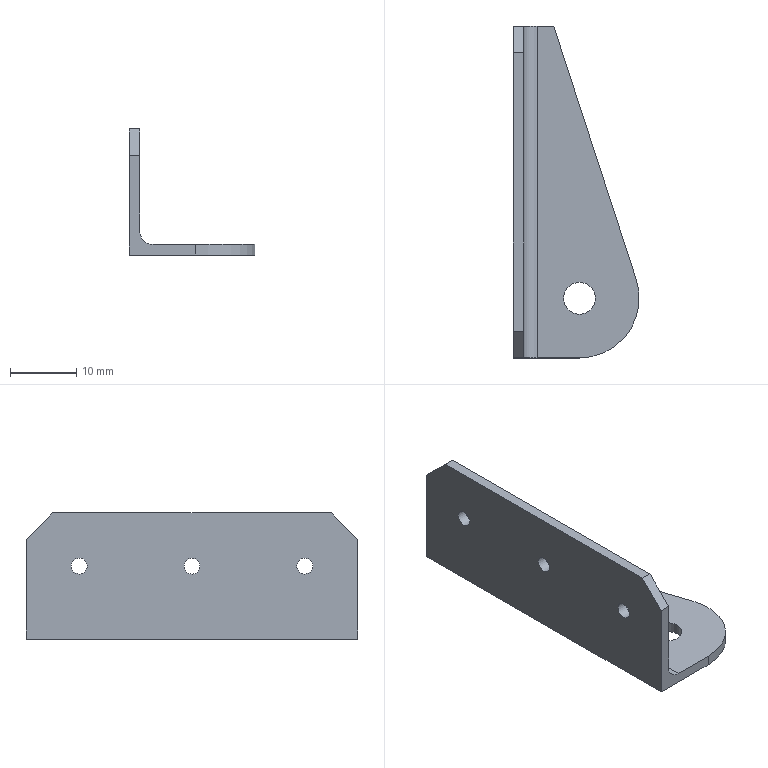Part | NX | features solid 2 | 1 solid | 16 faces | box 18.999 x 50 x 19 mm | volume 2444 mm3 | plane 10 | cylinder 6 | commonest cylinder face diameters 2.4 x3 4 x1 4.8 x1 17.997 x1
STEP:
#1=CARTESIAN_POINT('',(108.762,-251.916,9.8));
#2=VERTEX_POINT('',#1);
#3=CARTESIAN_POINT('',(108.762,-251.916,11.));
#4=DIRECTION('',(1.,0.,0.));
#5=DIRECTION('',(0.,0.,-1.));
#6=AXIS2_PLACEMENT_3D('',#3,#4,#5);
#7=CIRCLE('',#6,1.2);
#8=EDGE_CURVE('',#2,#2,#7,.F.);
#9=ORIENTED_EDGE('',*,*,#8,.F.);
#10=EDGE_LOOP('',(#9));
#11=FACE_BOUND('',#10,.T.);
#12=CARTESIAN_POINT('',(108.762,-259.916,15.));
#13=VERTEX_POINT('',#12);
#14=CARTESIAN_POINT('',(108.762,-259.916,0.));
#15=VERTEX_POINT('',#14);
#16=CARTESIAN_POINT('',(108.762,-259.916,19.));
#17=DIRECTION('',(0.,0.,-1.));
#18=VECTOR('',#17,1000.);
#19=LINE('',#16,#18);
#20=EDGE_CURVE('',#13,#15,#19,.T.);
#21=ORIENTED_EDGE('',*,*,#20,.F.);
#22=CARTESIAN_POINT('',(108.762,-255.916,19.));
#23=VERTEX_POINT('',#22);
#24=CARTESIAN_POINT('',(108.762,-255.916,19.));
#25=DIRECTION('',(0.,0.7071,0.7071));
#26=VECTOR('',#25,1000.);
#27=LINE('',#24,#26);
#28=EDGE_CURVE('',#13,#23,#27,.T.);
#29=ORIENTED_EDGE('',*,*,#28,.T.);
#30=CARTESIAN_POINT('',(108.762,-213.916,19.));
#31=VERTEX_POINT('',#30);
#32=CARTESIAN_POINT('',(108.762,-209.916,19.));
#33=DIRECTION('',(0.,-1.,0.));
#34=VECTOR('',#33,1000.);
#35=LINE('',#32,#34);
#36=EDGE_CURVE('',#31,#23,#35,.T.);
#37=ORIENTED_EDGE('',*,*,#36,.F.);
#38=CARTESIAN_POINT('',(108.762,-209.916,15.));
#39=VERTEX_POINT('',#38);
#40=CARTESIAN_POINT('',(108.762,-213.916,19.));
#41=DIRECTION('',(0.,0.7071,-0.7071));
#42=VECTOR('',#41,1000.);
#43=LINE('',#40,#42);
#44=EDGE_CURVE('',#31,#39,#43,.T.);
#45=ORIENTED_EDGE('',*,*,#44,.T.);
#46=CARTESIAN_POINT('',(108.762,-209.916,0.));
#47=VERTEX_POINT('',#46);
#48=CARTESIAN_POINT('',(108.762,-209.916,19.));
#49=DIRECTION('',(0.,0.,-1.));
#50=VECTOR('',#49,1000.);
#51=LINE('',#48,#50);
#52=EDGE_CURVE('',#39,#47,#51,.T.);
#53=ORIENTED_EDGE('',*,*,#52,.T.);
#54=CARTESIAN_POINT('',(108.762,-255.916,0.));
#55=DIRECTION('',(0.,-1.,0.));
#56=VECTOR('',#55,1000.);
#57=LINE('',#54,#56);
#58=EDGE_CURVE('',#47,#15,#57,.T.);
#59=ORIENTED_EDGE('',*,*,#58,.T.);
#60=EDGE_LOOP('',(#21,#29,#37,#45,#53,#59));
#61=FACE_BOUND('',#60,.T.);
#62=CARTESIAN_POINT('',(108.762,-234.916,9.8));
#63=VERTEX_POINT('',#62);
#64=CARTESIAN_POINT('',(108.762,-234.916,11.));
#65=DIRECTION('',(1.,0.,0.));
#66=DIRECTION('',(0.,0.,-1.));
#67=AXIS2_PLACEMENT_3D('',#64,#65,#66);
#68=CIRCLE('',#67,1.2);
#69=EDGE_CURVE('',#63,#63,#68,.F.);
#70=ORIENTED_EDGE('',*,*,#69,.F.);
#71=EDGE_LOOP('',(#70));
#72=FACE_BOUND('',#71,.T.);
#73=CARTESIAN_POINT('',(108.762,-217.916,9.8));
#74=VERTEX_POINT('',#73);
#75=CARTESIAN_POINT('',(108.762,-217.916,11.));
#76=DIRECTION('',(1.,0.,0.));
#77=DIRECTION('',(0.,0.,-1.));
#78=AXIS2_PLACEMENT_3D('',#75,#76,#77);
#79=CIRCLE('',#78,1.2);
#80=EDGE_CURVE('',#74,#74,#79,.F.);
#81=ORIENTED_EDGE('',*,*,#80,.F.);
#82=EDGE_LOOP('',(#81));
#83=FACE_BOUND('',#82,.T.);
#84=CARTESIAN_POINT('',(108.762,-255.916,19.));
#85=DIRECTION('',(1.,0.,0.));
#86=DIRECTION('',(0.,0.,-1.));
#87=AXIS2_PLACEMENT_3D('',#84,#85,#86);
#88=PLANE('',#87);
#89=ADVANCED_FACE('',(#11,#61,#72,#83),#88,.F.);
#90=CARTESIAN_POINT('',(110.362,-251.916,9.8));
#91=VERTEX_POINT('',#90);
#92=CARTESIAN_POINT('',(110.362,-251.916,11.));
#93=DIRECTION('',(1.,0.,0.));
#94=DIRECTION('',(0.,0.,-1.));
#95=AXIS2_PLACEMENT_3D('',#92,#93,#94);
#96=CIRCLE('',#95,1.2);
#97=EDGE_CURVE('',#91,#91,#96,.F.);
#98=ORIENTED_EDGE('',*,*,#97,.T.);
#99=EDGE_LOOP('',(#98));
#100=FACE_BOUND('',#99,.T.);
#101=CARTESIAN_POINT('',(110.362,-259.916,15.));
#102=VERTEX_POINT('',#101);
#103=CARTESIAN_POINT('',(110.362,-259.916,3.6));
#104=VERTEX_POINT('',#103);
#105=CARTESIAN_POINT('',(110.362,-259.916,19.));
#106=DIRECTION('',(0.,0.,-1.));
#107=VECTOR('',#106,1000.);
#108=LINE('',#105,#107);
#109=EDGE_CURVE('',#102,#104,#108,.T.);
#110=ORIENTED_EDGE('',*,*,#109,.T.);
#111=CARTESIAN_POINT('',(110.362,-209.916,3.6));
#112=VERTEX_POINT('',#111);
#113=CARTESIAN_POINT('',(110.362,-209.916,3.6));
#114=DIRECTION('',(0.,-1.,0.));
#115=VECTOR('',#114,1000.);
#116=LINE('',#113,#115);
#117=EDGE_CURVE('',#104,#112,#116,.F.);
#118=ORIENTED_EDGE('',*,*,#117,.T.);
#119=CARTESIAN_POINT('',(110.362,-209.916,15.));
#120=VERTEX_POINT('',#119);
#121=CARTESIAN_POINT('',(110.362,-209.916,19.));
#122=DIRECTION('',(0.,0.,-1.));
#123=VECTOR('',#122,1000.);
#124=LINE('',#121,#123);
#125=EDGE_CURVE('',#120,#112,#124,.T.);
#126=ORIENTED_EDGE('',*,*,#125,.F.);
#127=CARTESIAN_POINT('',(110.362,-213.916,19.));
#128=VERTEX_POINT('',#127);
#129=CARTESIAN_POINT('',(110.362,-234.916,40.));
#130=DIRECTION('',(0.,-0.7071,0.7071));
#131=VECTOR('',#130,1000.);
#132=LINE('',#129,#131);
#133=EDGE_CURVE('',#120,#128,#132,.T.);
#134=ORIENTED_EDGE('',*,*,#133,.T.);
#135=CARTESIAN_POINT('',(110.362,-255.916,19.));
#136=VERTEX_POINT('',#135);
#137=CARTESIAN_POINT('',(110.362,-255.916,19.));
#138=DIRECTION('',(0.,-1.,0.));
#139=VECTOR('',#138,1000.);
#140=LINE('',#137,#139);
#141=EDGE_CURVE('',#128,#136,#140,.T.);
#142=ORIENTED_EDGE('',*,*,#141,.T.);
#143=CARTESIAN_POINT('',(110.362,-255.916,19.));
#144=DIRECTION('',(0.,-0.7071,-0.7071));
#145=VECTOR('',#144,1000.);
#146=LINE('',#143,#145);
#147=EDGE_CURVE('',#136,#102,#146,.T.);
#148=ORIENTED_EDGE('',*,*,#147,.T.);
#149=EDGE_LOOP('',(#110,#118,#126,#134,#142,#148));
#150=FACE_BOUND('',#149,.T.);
#151=CARTESIAN_POINT('',(110.362,-234.916,9.8));
#152=VERTEX_POINT('',#151);
#153=CARTESIAN_POINT('',(110.362,-234.916,11.));
#154=DIRECTION('',(1.,0.,0.));
#155=DIRECTION('',(0.,0.,-1.));
#156=AXIS2_PLACEMENT_3D('',#153,#154,#155);
#157=CIRCLE('',#156,1.2);
#158=EDGE_CURVE('',#152,#152,#157,.F.);
#159=ORIENTED_EDGE('',*,*,#158,.T.);
#160=EDGE_LOOP('',(#159));
#161=FACE_BOUND('',#160,.T.);
#162=CARTESIAN_POINT('',(110.362,-217.916,9.8));
#163=VERTEX_POINT('',#162);
#164=CARTESIAN_POINT('',(110.362,-217.916,11.));
#165=DIRECTION('',(1.,0.,0.));
#166=DIRECTION('',(0.,0.,-1.));
#167=AXIS2_PLACEMENT_3D('',#164,#165,#166);
#168=CIRCLE('',#167,1.2);
#169=EDGE_CURVE('',#163,#163,#168,.F.);
#170=ORIENTED_EDGE('',*,*,#169,.T.);
#171=EDGE_LOOP('',(#170));
#172=FACE_BOUND('',#171,.T.);
#173=CARTESIAN_POINT('',(110.362,-255.916,19.));
#174=DIRECTION('',(1.,0.,0.));
#175=DIRECTION('',(0.,0.,-1.));
#176=AXIS2_PLACEMENT_3D('',#173,#174,#175);
#177=PLANE('',#176);
#178=ADVANCED_FACE('',(#100,#150,#161,#172),#177,.T.);
#179=ORIENTED_EDGE('',*,*,#52,.F.);
#180=CARTESIAN_POINT('',(110.362,-209.916,15.));
#181=DIRECTION('',(1.,0.,0.));
#182=VECTOR('',#181,1000.);
#183=LINE('',#180,#182);
#184=EDGE_CURVE('',#39,#120,#183,.T.);
#185=ORIENTED_EDGE('',*,*,#184,.T.);
#186=ORIENTED_EDGE('',*,*,#125,.T.);
#187=CARTESIAN_POINT('',(112.362,-209.916,1.6));
#188=VERTEX_POINT('',#187);
#189=CARTESIAN_POINT('',(112.362,-209.916,3.6));
#190=DIRECTION('',(0.,-1.,0.));
#191=DIRECTION('',(0.,0.,-1.));
#192=AXIS2_PLACEMENT_3D('',#189,#190,#191);
#193=CIRCLE('',#192,2.);
#194=EDGE_CURVE('',#112,#188,#193,.T.);
#195=ORIENTED_EDGE('',*,*,#194,.T.);
#196=CARTESIAN_POINT('',(114.893,-209.916,1.6));
#197=VERTEX_POINT('',#196);
#198=CARTESIAN_POINT('',(110.362,-209.916,1.6));
#199=DIRECTION('',(-1.,0.,0.));
#200=VECTOR('',#199,1000.);
#201=LINE('',#198,#200);
#202=EDGE_CURVE('',#197,#188,#201,.T.);
#203=ORIENTED_EDGE('',*,*,#202,.F.);
#204=CARTESIAN_POINT('',(114.893,-209.916,0.));
#205=VERTEX_POINT('',#204);
#206=CARTESIAN_POINT('',(114.893,-209.916,19.));
#207=DIRECTION('',(0.,0.,-1.));
#208=VECTOR('',#207,1000.);
#209=LINE('',#206,#208);
#210=EDGE_CURVE('',#197,#205,#209,.T.);
#211=ORIENTED_EDGE('',*,*,#210,.T.);
#212=CARTESIAN_POINT('',(110.362,-209.916,0.));
#213=DIRECTION('',(-1.,0.,0.));
#214=VECTOR('',#213,1000.);
#215=LINE('',#212,#214);
#216=EDGE_CURVE('',#205,#47,#215,.T.);
#217=ORIENTED_EDGE('',*,*,#216,.T.);
#218=EDGE_LOOP('',(#179,#185,#186,#195,#203,#211,#217));
#219=FACE_BOUND('',#218,.T.);
#220=CARTESIAN_POINT('',(110.362,-209.916,19.));
#221=DIRECTION('',(0.,-1.,0.));
#222=DIRECTION('',(0.,0.,-1.));
#223=AXIS2_PLACEMENT_3D('',#220,#221,#222);
#224=PLANE('',#223);
#225=ADVANCED_FACE('',(#219),#224,.F.);
#226=ORIENTED_EDGE('',*,*,#109,.F.);
#227=CARTESIAN_POINT('',(108.762,-259.916,15.));
#228=DIRECTION('',(-1.,0.,0.));
#229=VECTOR('',#228,1000.);
#230=LINE('',#227,#229);
#231=EDGE_CURVE('',#102,#13,#230,.T.);
#232=ORIENTED_EDGE('',*,*,#231,.T.);
#233=ORIENTED_EDGE('',*,*,#20,.T.);
#234=CARTESIAN_POINT('',(118.762,-259.916,0.));
#235=VERTEX_POINT('',#234);
#236=CARTESIAN_POINT('',(112.362,-259.916,0.));
#237=DIRECTION('',(1.,0.,0.));
#238=VECTOR('',#237,1000.);
#239=LINE('',#236,#238);
#240=EDGE_CURVE('',#15,#235,#239,.T.);
#241=ORIENTED_EDGE('',*,*,#240,.T.);
#242=CARTESIAN_POINT('',(118.762,-259.916,1.6));
#243=VERTEX_POINT('',#242);
#244=CARTESIAN_POINT('',(118.762,-259.916,19.));
#245=DIRECTION('',(0.,0.,-1.));
#246=VECTOR('',#245,1000.);
#247=LINE('',#244,#246);
#248=EDGE_CURVE('',#243,#235,#247,.T.);
#249=ORIENTED_EDGE('',*,*,#248,.F.);
#250=CARTESIAN_POINT('',(112.362,-259.916,1.6));
#251=VERTEX_POINT('',#250);
#252=CARTESIAN_POINT('',(112.362,-259.916,1.6));
#253=DIRECTION('',(1.,0.,0.));
#254=VECTOR('',#253,1000.);
#255=LINE('',#252,#254);
#256=EDGE_CURVE('',#251,#243,#255,.T.);
#257=ORIENTED_EDGE('',*,*,#256,.F.);
#258=CARTESIAN_POINT('',(112.362,-259.916,3.6));
#259=DIRECTION('',(0.,1.,0.));
#260=DIRECTION('',(0.,0.,1.));
#261=AXIS2_PLACEMENT_3D('',#258,#259,#260);
#262=CIRCLE('',#261,2.);
#263=EDGE_CURVE('',#251,#104,#262,.T.);
#264=ORIENTED_EDGE('',*,*,#263,.T.);
#265=EDGE_LOOP('',(#226,#232,#233,#241,#249,#257,#264));
#266=FACE_BOUND('',#265,.T.);
#267=CARTESIAN_POINT('',(112.362,-259.916,19.));
#268=DIRECTION('',(0.,1.,0.));
#269=DIRECTION('',(0.,0.,1.));
#270=AXIS2_PLACEMENT_3D('',#267,#268,#269);
#271=PLANE('',#270);
#272=ADVANCED_FACE('',(#266),#271,.F.);
#273=CARTESIAN_POINT('',(127.32,-248.135,1.6));
#274=VERTEX_POINT('',#273);
#275=CARTESIAN_POINT('',(118.762,-250.917,1.6));
#276=DIRECTION('',(0.,0.,1.));
#277=DIRECTION('',(1.,0.,0.));
#278=AXIS2_PLACEMENT_3D('',#275,#276,#277);
#279=CIRCLE('',#278,8.999);
#280=EDGE_CURVE('',#243,#274,#279,.T.);
#281=ORIENTED_EDGE('',*,*,#280,.F.);
#282=ORIENTED_EDGE('',*,*,#248,.T.);
#283=CARTESIAN_POINT('',(127.32,-248.135,0.));
#284=VERTEX_POINT('',#283);
#285=CARTESIAN_POINT('',(118.762,-250.917,0.));
#286=DIRECTION('',(0.,0.,1.));
#287=DIRECTION('',(1.,0.,0.));
#288=AXIS2_PLACEMENT_3D('',#285,#286,#287);
#289=CIRCLE('',#288,8.999);
#290=EDGE_CURVE('',#235,#284,#289,.T.);
#291=ORIENTED_EDGE('',*,*,#290,.T.);
#292=CARTESIAN_POINT('',(127.32,-248.135,19.));
#293=DIRECTION('',(0.,0.,-1.));
#294=VECTOR('',#293,1000.);
#295=LINE('',#292,#294);
#296=EDGE_CURVE('',#274,#284,#295,.T.);
#297=ORIENTED_EDGE('',*,*,#296,.F.);
#298=EDGE_LOOP('',(#281,#282,#291,#297));
#299=FACE_BOUND('',#298,.T.);
#300=CARTESIAN_POINT('',(118.762,-250.917,19.));
#301=DIRECTION('',(0.,0.,-1.));
#302=DIRECTION('',(-1.,0.,0.));
#303=AXIS2_PLACEMENT_3D('',#300,#301,#302);
#304=CYLINDRICAL_SURFACE('',#303,8.999);
#305=ADVANCED_FACE('',(#299),#304,.T.);
#306=CARTESIAN_POINT('',(127.32,-248.135,1.6));
#307=DIRECTION('',(-0.3092,0.951,0.));
#308=VECTOR('',#307,1000.);
#309=LINE('',#306,#308);
#310=EDGE_CURVE('',#274,#197,#309,.T.);
#311=ORIENTED_EDGE('',*,*,#310,.F.);
#312=ORIENTED_EDGE('',*,*,#296,.T.);
#313=CARTESIAN_POINT('',(127.32,-248.135,0.));
#314=DIRECTION('',(-0.3092,0.951,0.));
#315=VECTOR('',#314,1000.);
#316=LINE('',#313,#315);
#317=EDGE_CURVE('',#284,#205,#316,.T.);
#318=ORIENTED_EDGE('',*,*,#317,.T.);
#319=ORIENTED_EDGE('',*,*,#210,.F.);
#320=EDGE_LOOP('',(#311,#312,#318,#319));
#321=FACE_BOUND('',#320,.T.);
#322=CARTESIAN_POINT('',(127.32,-248.135,19.));
#323=DIRECTION('',(-0.951,-0.3092,0.));
#324=DIRECTION('',(0.3092,-0.951,0.));
#325=AXIS2_PLACEMENT_3D('',#322,#323,#324);
#326=PLANE('',#325);
#327=ADVANCED_FACE('',(#321),#326,.F.);
#328=CARTESIAN_POINT('',(121.162,-250.917,0.));
#329=VERTEX_POINT('',#328);
#330=CARTESIAN_POINT('',(118.762,-250.917,0.));
#331=DIRECTION('',(0.,0.,1.));
#332=DIRECTION('',(1.,0.,0.));
#333=AXIS2_PLACEMENT_3D('',#330,#331,#332);
#334=CIRCLE('',#333,2.4);
#335=EDGE_CURVE('',#329,#329,#334,.T.);
#336=ORIENTED_EDGE('',*,*,#335,.F.);
#337=EDGE_LOOP('',(#336));
#338=FACE_BOUND('',#337,.T.);
#339=CARTESIAN_POINT('',(121.162,-250.917,1.6));
#340=VERTEX_POINT('',#339);
#341=CARTESIAN_POINT('',(118.762,-250.917,1.6));
#342=DIRECTION('',(0.,0.,1.));
#343=DIRECTION('',(1.,0.,0.));
#344=AXIS2_PLACEMENT_3D('',#341,#342,#343);
#345=CIRCLE('',#344,2.4);
#346=EDGE_CURVE('',#340,#340,#345,.T.);
#347=ORIENTED_EDGE('',*,*,#346,.T.);
#348=EDGE_LOOP('',(#347));
#349=FACE_BOUND('',#348,.T.);
#350=CARTESIAN_POINT('',(118.762,-250.917,19.));
#351=DIRECTION('',(0.,0.,-1.));
#352=DIRECTION('',(-1.,0.,0.));
#353=AXIS2_PLACEMENT_3D('',#350,#351,#352);
#354=CYLINDRICAL_SURFACE('',#353,2.4);
#355=ADVANCED_FACE('',(#338,#349),#354,.F.);
#356=ORIENTED_EDGE('',*,*,#36,.T.);
#357=CARTESIAN_POINT('',(110.362,-255.916,19.));
#358=DIRECTION('',(1.,0.,0.));
#359=VECTOR('',#358,1000.);
#360=LINE('',#357,#359);
#361=EDGE_CURVE('',#23,#136,#360,.T.);
#362=ORIENTED_EDGE('',*,*,#361,.T.);
#363=ORIENTED_EDGE('',*,*,#141,.F.);
#364=CARTESIAN_POINT('',(108.762,-213.916,19.));
#365=DIRECTION('',(-1.,0.,0.));
#366=VECTOR('',#365,1000.);
#367=LINE('',#364,#366);
#368=EDGE_CURVE('',#128,#31,#367,.T.);
#369=ORIENTED_EDGE('',*,*,#368,.T.);
#370=EDGE_LOOP('',(#356,#362,#363,#369));
#371=FACE_BOUND('',#370,.T.);
#372=CARTESIAN_POINT('',(118.762,-250.917,19.));
#373=DIRECTION('',(0.,0.,1.));
#374=DIRECTION('',(1.,0.,0.));
#375=AXIS2_PLACEMENT_3D('',#372,#373,#374);
#376=PLANE('',#375);
#377=ADVANCED_FACE('',(#371),#376,.T.);
#378=ORIENTED_EDGE('',*,*,#216,.F.);
#379=ORIENTED_EDGE('',*,*,#317,.F.);
#380=ORIENTED_EDGE('',*,*,#290,.F.);
#381=ORIENTED_EDGE('',*,*,#240,.F.);
#382=ORIENTED_EDGE('',*,*,#58,.F.);
#383=EDGE_LOOP('',(#378,#379,#380,#381,#382));
#384=FACE_BOUND('',#383,.T.);
#385=ORIENTED_EDGE('',*,*,#335,.T.);
#386=EDGE_LOOP('',(#385));
#387=FACE_BOUND('',#386,.T.);
#388=CARTESIAN_POINT('',(118.762,-250.917,0.));
#389=DIRECTION('',(0.,0.,1.));
#390=DIRECTION('',(1.,0.,0.));
#391=AXIS2_PLACEMENT_3D('',#388,#389,#390);
#392=PLANE('',#391);
#393=ADVANCED_FACE('',(#384,#387),#392,.F.);
#394=ORIENTED_EDGE('',*,*,#202,.T.);
#395=CARTESIAN_POINT('',(112.362,-259.916,1.6));
#396=DIRECTION('',(0.,-1.,0.));
#397=VECTOR('',#396,1000.);
#398=LINE('',#395,#397);
#399=EDGE_CURVE('',#188,#251,#398,.T.);
#400=ORIENTED_EDGE('',*,*,#399,.T.);
#401=ORIENTED_EDGE('',*,*,#256,.T.);
#402=ORIENTED_EDGE('',*,*,#280,.T.);
#403=ORIENTED_EDGE('',*,*,#310,.T.);
#404=EDGE_LOOP('',(#394,#400,#401,#402,#403));
#405=FACE_BOUND('',#404,.T.);
#406=ORIENTED_EDGE('',*,*,#346,.F.);
#407=EDGE_LOOP('',(#406));
#408=FACE_BOUND('',#407,.T.);
#409=CARTESIAN_POINT('',(118.762,-250.917,1.6));
#410=DIRECTION('',(0.,0.,1.));
#411=DIRECTION('',(1.,0.,0.));
#412=AXIS2_PLACEMENT_3D('',#409,#410,#411);
#413=PLANE('',#412);
#414=ADVANCED_FACE('',(#405,#408),#413,.T.);
#415=ORIENTED_EDGE('',*,*,#28,.F.);
#416=ORIENTED_EDGE('',*,*,#231,.F.);
#417=ORIENTED_EDGE('',*,*,#147,.F.);
#418=ORIENTED_EDGE('',*,*,#361,.F.);
#419=EDGE_LOOP('',(#415,#416,#417,#418));
#420=FACE_BOUND('',#419,.T.);
#421=CARTESIAN_POINT('',(118.762,-255.916,19.));
#422=DIRECTION('',(0.,-0.7071,0.7071));
#423=DIRECTION('',(-1.,0.,0.));
#424=AXIS2_PLACEMENT_3D('',#421,#422,#423);
#425=PLANE('',#424);
#426=ADVANCED_FACE('',(#420),#425,.T.);
#427=ORIENTED_EDGE('',*,*,#133,.F.);
#428=ORIENTED_EDGE('',*,*,#184,.F.);
#429=ORIENTED_EDGE('',*,*,#44,.F.);
#430=ORIENTED_EDGE('',*,*,#368,.F.);
#431=EDGE_LOOP('',(#427,#428,#429,#430));
#432=FACE_BOUND('',#431,.T.);
#433=CARTESIAN_POINT('',(118.762,-213.916,19.));
#434=DIRECTION('',(0.,0.7071,0.7071));
#435=DIRECTION('',(1.,0.,0.));
#436=AXIS2_PLACEMENT_3D('',#433,#434,#435);
#437=PLANE('',#436);
#438=ADVANCED_FACE('',(#432),#437,.T.);
#439=ORIENTED_EDGE('',*,*,#194,.F.);
#440=ORIENTED_EDGE('',*,*,#117,.F.);
#441=ORIENTED_EDGE('',*,*,#263,.F.);
#442=ORIENTED_EDGE('',*,*,#399,.F.);
#443=EDGE_LOOP('',(#439,#440,#441,#442));
#444=FACE_BOUND('',#443,.T.);
#445=CARTESIAN_POINT('',(112.362,-250.917,3.6));
#446=DIRECTION('',(0.,1.,0.));
#447=DIRECTION('',(0.,0.,1.));
#448=AXIS2_PLACEMENT_3D('',#445,#446,#447);
#449=CYLINDRICAL_SURFACE('',#448,2.);
#450=ADVANCED_FACE('',(#444),#449,.F.);
#451=ORIENTED_EDGE('',*,*,#158,.F.);
#452=EDGE_LOOP('',(#451));
#453=FACE_BOUND('',#452,.T.);
#454=ORIENTED_EDGE('',*,*,#69,.T.);
#455=EDGE_LOOP('',(#454));
#456=FACE_BOUND('',#455,.T.);
#457=CARTESIAN_POINT('',(89.762,-234.916,11.));
#458=DIRECTION('',(1.,0.,0.));
#459=DIRECTION('',(0.,0.,-1.));
#460=AXIS2_PLACEMENT_3D('',#457,#458,#459);
#461=CYLINDRICAL_SURFACE('',#460,1.2);
#462=ADVANCED_FACE('',(#453,#456),#461,.F.);
#463=ORIENTED_EDGE('',*,*,#97,.F.);
#464=EDGE_LOOP('',(#463));
#465=FACE_BOUND('',#464,.T.);
#466=ORIENTED_EDGE('',*,*,#8,.T.);
#467=EDGE_LOOP('',(#466));
#468=FACE_BOUND('',#467,.T.);
#469=CARTESIAN_POINT('',(89.762,-251.916,11.));
#470=DIRECTION('',(1.,0.,0.));
#471=DIRECTION('',(0.,0.,-1.));
#472=AXIS2_PLACEMENT_3D('',#469,#470,#471);
#473=CYLINDRICAL_SURFACE('',#472,1.2);
#474=ADVANCED_FACE('',(#465,#468),#473,.F.);
#475=ORIENTED_EDGE('',*,*,#169,.F.);
#476=EDGE_LOOP('',(#475));
#477=FACE_BOUND('',#476,.T.);
#478=ORIENTED_EDGE('',*,*,#80,.T.);
#479=EDGE_LOOP('',(#478));
#480=FACE_BOUND('',#479,.T.);
#481=CARTESIAN_POINT('',(89.762,-217.916,11.));
#482=DIRECTION('',(1.,0.,0.));
#483=DIRECTION('',(0.,0.,-1.));
#484=AXIS2_PLACEMENT_3D('',#481,#482,#483);
#485=CYLINDRICAL_SURFACE('',#484,1.2);
#486=ADVANCED_FACE('',(#477,#480),#485,.F.);
#487=CLOSED_SHELL('',(#89,#178,#225,#272,#305,#327,#355,#377,#393,#414,#426,#438,#450,#462,#474,#486));
#488=MANIFOLD_SOLID_BREP('',#487);
#489=(LENGTH_UNIT()NAMED_UNIT(*)SI_UNIT(.MILLI.,.METRE.));
#490=UNCERTAINTY_MEASURE_WITH_UNIT(LENGTH_MEASURE(0.00001),#489,'','');
#491=(NAMED_UNIT(*)PLANE_ANGLE_UNIT()SI_UNIT($,.RADIAN.));
#492=(NAMED_UNIT(*)SI_UNIT($,.STERADIAN.)SOLID_ANGLE_UNIT());
#493=(GEOMETRIC_REPRESENTATION_CONTEXT(3)GLOBAL_UNCERTAINTY_ASSIGNED_CONTEXT((#490))GLOBAL_UNIT_ASSIGNED_CONTEXT((#489,#491,#492))REPRESENTATION_CONTEXT('',''));
#494=ADVANCED_BREP_SHAPE_REPRESENTATION('',(#488),#493);